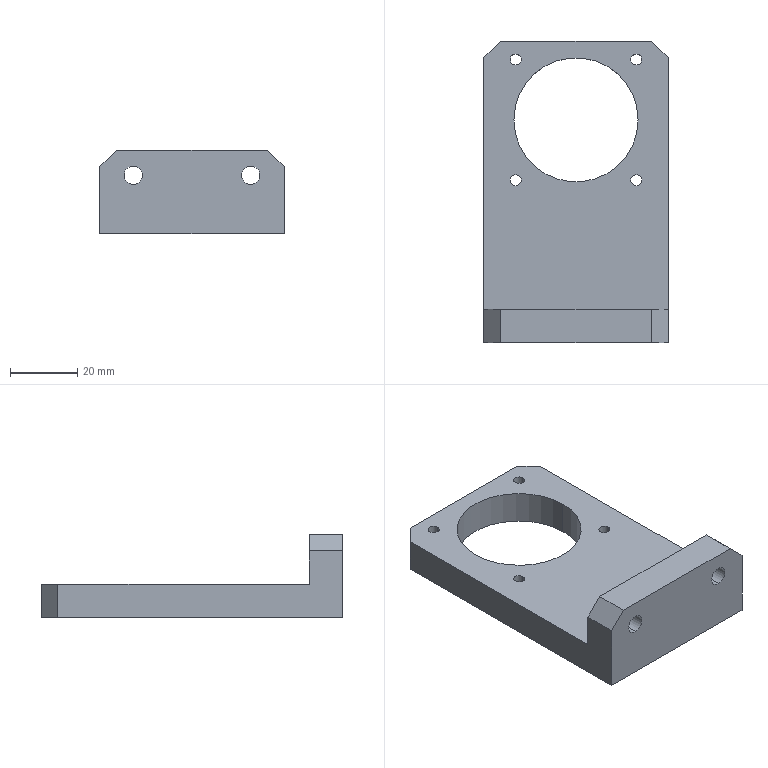Part | NX | features BREP 1 | 1 solid | 26 faces | box 55 x 90 x 25 mm | volume 45681 mm3 | cylinder 14 | plane 12 | commonest cylinder face diameters 3.3 x8 5.5 x4 37 x2
STEP:
#1=CARTESIAN_POINT('',(17.347,3.533,10.));
#2=VERTEX_POINT('',#1);
#3=CARTESIAN_POINT('',(-19.653,3.533,10.));
#4=VERTEX_POINT('',#3);
#5=CARTESIAN_POINT('',(-1.153,3.533,10.));
#6=DIRECTION('',(0.,0.,-1.));
#7=DIRECTION('',(-1.,0.,0.));
#8=AXIS2_PLACEMENT_3D('',#5,#6,#7);
#9=CIRCLE('',#8,18.5);
#10=EDGE_CURVE('',#2,#4,#9,.T.);
#11=ORIENTED_EDGE('',*,*,#10,.F.);
#12=CARTESIAN_POINT('',(17.347,3.533,0.));
#13=VERTEX_POINT('',#12);
#14=CARTESIAN_POINT('',(17.347,3.533,25.));
#15=DIRECTION('',(0.,0.,-1.));
#16=VECTOR('',#15,1000.);
#17=LINE('',#14,#16);
#18=EDGE_CURVE('',#2,#13,#17,.T.);
#19=ORIENTED_EDGE('',*,*,#18,.T.);
#20=CARTESIAN_POINT('',(-19.653,3.533,0.));
#21=VERTEX_POINT('',#20);
#22=CARTESIAN_POINT('',(-1.153,3.533,0.));
#23=DIRECTION('',(0.,0.,-1.));
#24=DIRECTION('',(-1.,0.,0.));
#25=AXIS2_PLACEMENT_3D('',#22,#23,#24);
#26=CIRCLE('',#25,18.5);
#27=EDGE_CURVE('',#13,#21,#26,.T.);
#28=ORIENTED_EDGE('',*,*,#27,.T.);
#29=CARTESIAN_POINT('',(-19.653,3.533,25.));
#30=DIRECTION('',(0.,0.,-1.));
#31=VECTOR('',#30,1000.);
#32=LINE('',#29,#31);
#33=EDGE_CURVE('',#4,#21,#32,.T.);
#34=ORIENTED_EDGE('',*,*,#33,.F.);
#35=EDGE_LOOP('',(#11,#19,#28,#34));
#36=FACE_BOUND('',#35,.T.);
#37=CARTESIAN_POINT('',(-1.153,3.533,25.));
#38=DIRECTION('',(0.,0.,-1.));
#39=DIRECTION('',(-1.,0.,0.));
#40=AXIS2_PLACEMENT_3D('',#37,#38,#39);
#41=CYLINDRICAL_SURFACE('',#40,18.5);
#42=ADVANCED_FACE('',(#36),#41,.F.);
#43=CARTESIAN_POINT('',(18.497,-14.467,0.));
#44=VERTEX_POINT('',#43);
#45=CARTESIAN_POINT('',(15.197,-14.467,0.));
#46=VERTEX_POINT('',#45);
#47=CARTESIAN_POINT('',(16.847,-14.467,0.));
#48=DIRECTION('',(0.,0.,-1.));
#49=DIRECTION('',(1.,0.,0.));
#50=AXIS2_PLACEMENT_3D('',#47,#48,#49);
#51=CIRCLE('',#50,1.65);
#52=EDGE_CURVE('',#44,#46,#51,.T.);
#53=ORIENTED_EDGE('',*,*,#52,.T.);
#54=CARTESIAN_POINT('',(15.197,-14.467,10.));
#55=VERTEX_POINT('',#54);
#56=CARTESIAN_POINT('',(15.197,-14.467,10.));
#57=DIRECTION('',(0.,0.,1.));
#58=VECTOR('',#57,1000.);
#59=LINE('',#56,#58);
#60=EDGE_CURVE('',#55,#46,#59,.F.);
#61=ORIENTED_EDGE('',*,*,#60,.F.);
#62=CARTESIAN_POINT('',(18.497,-14.467,10.));
#63=VERTEX_POINT('',#62);
#64=CARTESIAN_POINT('',(16.847,-14.467,10.));
#65=DIRECTION('',(0.,0.,-1.));
#66=DIRECTION('',(1.,0.,0.));
#67=AXIS2_PLACEMENT_3D('',#64,#65,#66);
#68=CIRCLE('',#67,1.65);
#69=EDGE_CURVE('',#63,#55,#68,.T.);
#70=ORIENTED_EDGE('',*,*,#69,.F.);
#71=CARTESIAN_POINT('',(18.497,-14.467,10.));
#72=DIRECTION('',(0.,0.,1.));
#73=VECTOR('',#72,1000.);
#74=LINE('',#71,#73);
#75=EDGE_CURVE('',#63,#44,#74,.F.);
#76=ORIENTED_EDGE('',*,*,#75,.T.);
#77=EDGE_LOOP('',(#53,#61,#70,#76));
#78=FACE_BOUND('',#77,.T.);
#79=CARTESIAN_POINT('',(16.847,-14.467,10.));
#80=DIRECTION('',(0.,0.,1.));
#81=DIRECTION('',(1.,0.,0.));
#82=AXIS2_PLACEMENT_3D('',#79,#80,#81);
#83=CYLINDRICAL_SURFACE('',#82,1.65);
#84=ADVANCED_FACE('',(#78),#83,.F.);
#85=CARTESIAN_POINT('',(18.497,21.533,0.));
#86=VERTEX_POINT('',#85);
#87=CARTESIAN_POINT('',(15.197,21.533,0.));
#88=VERTEX_POINT('',#87);
#89=CARTESIAN_POINT('',(16.847,21.533,0.));
#90=DIRECTION('',(0.,0.,-1.));
#91=DIRECTION('',(1.,0.,0.));
#92=AXIS2_PLACEMENT_3D('',#89,#90,#91);
#93=CIRCLE('',#92,1.65);
#94=EDGE_CURVE('',#86,#88,#93,.T.);
#95=ORIENTED_EDGE('',*,*,#94,.T.);
#96=CARTESIAN_POINT('',(15.197,21.533,10.));
#97=VERTEX_POINT('',#96);
#98=CARTESIAN_POINT('',(15.197,21.533,10.));
#99=DIRECTION('',(0.,0.,1.));
#100=VECTOR('',#99,1000.);
#101=LINE('',#98,#100);
#102=EDGE_CURVE('',#97,#88,#101,.F.);
#103=ORIENTED_EDGE('',*,*,#102,.F.);
#104=CARTESIAN_POINT('',(18.497,21.533,10.));
#105=VERTEX_POINT('',#104);
#106=CARTESIAN_POINT('',(16.847,21.533,10.));
#107=DIRECTION('',(0.,0.,-1.));
#108=DIRECTION('',(1.,0.,0.));
#109=AXIS2_PLACEMENT_3D('',#106,#107,#108);
#110=CIRCLE('',#109,1.65);
#111=EDGE_CURVE('',#105,#97,#110,.T.);
#112=ORIENTED_EDGE('',*,*,#111,.F.);
#113=CARTESIAN_POINT('',(18.497,21.533,10.));
#114=DIRECTION('',(0.,0.,1.));
#115=VECTOR('',#114,1000.);
#116=LINE('',#113,#115);
#117=EDGE_CURVE('',#105,#86,#116,.F.);
#118=ORIENTED_EDGE('',*,*,#117,.T.);
#119=EDGE_LOOP('',(#95,#103,#112,#118));
#120=FACE_BOUND('',#119,.T.);
#121=CARTESIAN_POINT('',(16.847,21.533,10.));
#122=DIRECTION('',(0.,0.,1.));
#123=DIRECTION('',(1.,0.,0.));
#124=AXIS2_PLACEMENT_3D('',#121,#122,#123);
#125=CYLINDRICAL_SURFACE('',#124,1.65);
#126=ADVANCED_FACE('',(#120),#125,.F.);
#127=CARTESIAN_POINT('',(-17.503,21.533,0.));
#128=VERTEX_POINT('',#127);
#129=CARTESIAN_POINT('',(-20.803,21.533,0.));
#130=VERTEX_POINT('',#129);
#131=CARTESIAN_POINT('',(-19.153,21.533,0.));
#132=DIRECTION('',(0.,0.,-1.));
#133=DIRECTION('',(1.,0.,0.));
#134=AXIS2_PLACEMENT_3D('',#131,#132,#133);
#135=CIRCLE('',#134,1.65);
#136=EDGE_CURVE('',#128,#130,#135,.T.);
#137=ORIENTED_EDGE('',*,*,#136,.T.);
#138=CARTESIAN_POINT('',(-20.803,21.533,10.));
#139=VERTEX_POINT('',#138);
#140=CARTESIAN_POINT('',(-20.803,21.533,10.));
#141=DIRECTION('',(0.,0.,1.));
#142=VECTOR('',#141,1000.);
#143=LINE('',#140,#142);
#144=EDGE_CURVE('',#139,#130,#143,.F.);
#145=ORIENTED_EDGE('',*,*,#144,.F.);
#146=CARTESIAN_POINT('',(-17.503,21.533,10.));
#147=VERTEX_POINT('',#146);
#148=CARTESIAN_POINT('',(-19.153,21.533,10.));
#149=DIRECTION('',(0.,0.,-1.));
#150=DIRECTION('',(1.,0.,0.));
#151=AXIS2_PLACEMENT_3D('',#148,#149,#150);
#152=CIRCLE('',#151,1.65);
#153=EDGE_CURVE('',#147,#139,#152,.T.);
#154=ORIENTED_EDGE('',*,*,#153,.F.);
#155=CARTESIAN_POINT('',(-17.503,21.533,10.));
#156=DIRECTION('',(0.,0.,1.));
#157=VECTOR('',#156,1000.);
#158=LINE('',#155,#157);
#159=EDGE_CURVE('',#147,#128,#158,.F.);
#160=ORIENTED_EDGE('',*,*,#159,.T.);
#161=EDGE_LOOP('',(#137,#145,#154,#160));
#162=FACE_BOUND('',#161,.T.);
#163=CARTESIAN_POINT('',(-19.153,21.533,10.));
#164=DIRECTION('',(0.,0.,1.));
#165=DIRECTION('',(1.,0.,0.));
#166=AXIS2_PLACEMENT_3D('',#163,#164,#165);
#167=CYLINDRICAL_SURFACE('',#166,1.65);
#168=ADVANCED_FACE('',(#162),#167,.F.);
#169=CARTESIAN_POINT('',(-17.503,-14.467,0.));
#170=VERTEX_POINT('',#169);
#171=CARTESIAN_POINT('',(-20.803,-14.467,0.));
#172=VERTEX_POINT('',#171);
#173=CARTESIAN_POINT('',(-19.153,-14.467,0.));
#174=DIRECTION('',(0.,0.,-1.));
#175=DIRECTION('',(1.,0.,0.));
#176=AXIS2_PLACEMENT_3D('',#173,#174,#175);
#177=CIRCLE('',#176,1.65);
#178=EDGE_CURVE('',#170,#172,#177,.T.);
#179=ORIENTED_EDGE('',*,*,#178,.T.);
#180=CARTESIAN_POINT('',(-20.803,-14.467,10.));
#181=VERTEX_POINT('',#180);
#182=CARTESIAN_POINT('',(-20.803,-14.467,10.));
#183=DIRECTION('',(0.,0.,1.));
#184=VECTOR('',#183,1000.);
#185=LINE('',#182,#184);
#186=EDGE_CURVE('',#181,#172,#185,.F.);
#187=ORIENTED_EDGE('',*,*,#186,.F.);
#188=CARTESIAN_POINT('',(-17.503,-14.467,10.));
#189=VERTEX_POINT('',#188);
#190=CARTESIAN_POINT('',(-19.153,-14.467,10.));
#191=DIRECTION('',(0.,0.,-1.));
#192=DIRECTION('',(1.,0.,0.));
#193=AXIS2_PLACEMENT_3D('',#190,#191,#192);
#194=CIRCLE('',#193,1.65);
#195=EDGE_CURVE('',#189,#181,#194,.T.);
#196=ORIENTED_EDGE('',*,*,#195,.F.);
#197=CARTESIAN_POINT('',(-17.503,-14.467,10.));
#198=DIRECTION('',(0.,0.,1.));
#199=VECTOR('',#198,1000.);
#200=LINE('',#197,#199);
#201=EDGE_CURVE('',#189,#170,#200,.F.);
#202=ORIENTED_EDGE('',*,*,#201,.T.);
#203=EDGE_LOOP('',(#179,#187,#196,#202));
#204=FACE_BOUND('',#203,.T.);
#205=CARTESIAN_POINT('',(-19.153,-14.467,10.));
#206=DIRECTION('',(0.,0.,1.));
#207=DIRECTION('',(1.,0.,0.));
#208=AXIS2_PLACEMENT_3D('',#205,#206,#207);
#209=CYLINDRICAL_SURFACE('',#208,1.65);
#210=ADVANCED_FACE('',(#204),#209,.F.);
#211=CARTESIAN_POINT('',(-18.653,-62.967,20.25));
#212=VERTEX_POINT('',#211);
#213=CARTESIAN_POINT('',(-18.653,-62.967,14.75));
#214=VERTEX_POINT('',#213);
#215=CARTESIAN_POINT('',(-18.653,-62.967,17.5));
#216=DIRECTION('',(0.,-1.,0.));
#217=DIRECTION('',(0.,0.,1.));
#218=AXIS2_PLACEMENT_3D('',#215,#216,#217);
#219=CIRCLE('',#218,2.75);
#220=EDGE_CURVE('',#212,#214,#219,.T.);
#221=ORIENTED_EDGE('',*,*,#220,.T.);
#222=CARTESIAN_POINT('',(-18.653,-52.967,14.75));
#223=VERTEX_POINT('',#222);
#224=CARTESIAN_POINT('',(-18.653,-62.967,14.75));
#225=DIRECTION('',(0.,1.,0.));
#226=VECTOR('',#225,1000.);
#227=LINE('',#224,#226);
#228=EDGE_CURVE('',#223,#214,#227,.F.);
#229=ORIENTED_EDGE('',*,*,#228,.F.);
#230=CARTESIAN_POINT('',(-18.653,-52.967,20.25));
#231=VERTEX_POINT('',#230);
#232=CARTESIAN_POINT('',(-18.653,-52.967,17.5));
#233=DIRECTION('',(0.,-1.,0.));
#234=DIRECTION('',(0.,0.,1.));
#235=AXIS2_PLACEMENT_3D('',#232,#233,#234);
#236=CIRCLE('',#235,2.75);
#237=EDGE_CURVE('',#231,#223,#236,.T.);
#238=ORIENTED_EDGE('',*,*,#237,.F.);
#239=CARTESIAN_POINT('',(-18.653,-62.967,20.25));
#240=DIRECTION('',(0.,1.,0.));
#241=VECTOR('',#240,1000.);
#242=LINE('',#239,#241);
#243=EDGE_CURVE('',#231,#212,#242,.F.);
#244=ORIENTED_EDGE('',*,*,#243,.T.);
#245=EDGE_LOOP('',(#221,#229,#238,#244));
#246=FACE_BOUND('',#245,.T.);
#247=CARTESIAN_POINT('',(-18.653,-62.967,17.5));
#248=DIRECTION('',(0.,1.,0.));
#249=DIRECTION('',(0.,0.,1.));
#250=AXIS2_PLACEMENT_3D('',#247,#248,#249);
#251=CYLINDRICAL_SURFACE('',#250,2.75);
#252=ADVANCED_FACE('',(#246),#251,.F.);
#253=CARTESIAN_POINT('',(16.347,-62.967,20.25));
#254=VERTEX_POINT('',#253);
#255=CARTESIAN_POINT('',(16.347,-62.967,14.75));
#256=VERTEX_POINT('',#255);
#257=CARTESIAN_POINT('',(16.347,-62.967,17.5));
#258=DIRECTION('',(0.,-1.,0.));
#259=DIRECTION('',(0.,0.,1.));
#260=AXIS2_PLACEMENT_3D('',#257,#258,#259);
#261=CIRCLE('',#260,2.75);
#262=EDGE_CURVE('',#254,#256,#261,.T.);
#263=ORIENTED_EDGE('',*,*,#262,.T.);
#264=CARTESIAN_POINT('',(16.347,-52.967,14.75));
#265=VERTEX_POINT('',#264);
#266=CARTESIAN_POINT('',(16.347,-62.967,14.75));
#267=DIRECTION('',(0.,1.,0.));
#268=VECTOR('',#267,1000.);
#269=LINE('',#266,#268);
#270=EDGE_CURVE('',#265,#256,#269,.F.);
#271=ORIENTED_EDGE('',*,*,#270,.F.);
#272=CARTESIAN_POINT('',(16.347,-52.967,20.25));
#273=VERTEX_POINT('',#272);
#274=CARTESIAN_POINT('',(16.347,-52.967,17.5));
#275=DIRECTION('',(0.,-1.,0.));
#276=DIRECTION('',(0.,0.,1.));
#277=AXIS2_PLACEMENT_3D('',#274,#275,#276);
#278=CIRCLE('',#277,2.75);
#279=EDGE_CURVE('',#273,#265,#278,.T.);
#280=ORIENTED_EDGE('',*,*,#279,.F.);
#281=CARTESIAN_POINT('',(16.347,-62.967,20.25));
#282=DIRECTION('',(0.,1.,0.));
#283=VECTOR('',#282,1000.);
#284=LINE('',#281,#283);
#285=EDGE_CURVE('',#273,#254,#284,.F.);
#286=ORIENTED_EDGE('',*,*,#285,.T.);
#287=EDGE_LOOP('',(#263,#271,#280,#286));
#288=FACE_BOUND('',#287,.T.);
#289=CARTESIAN_POINT('',(16.347,-62.967,17.5));
#290=DIRECTION('',(0.,1.,0.));
#291=DIRECTION('',(0.,0.,1.));
#292=AXIS2_PLACEMENT_3D('',#289,#290,#291);
#293=CYLINDRICAL_SURFACE('',#292,2.75);
#294=ADVANCED_FACE('',(#288),#293,.F.);
#295=CARTESIAN_POINT('',(26.347,22.033,0.));
#296=VERTEX_POINT('',#295);
#297=CARTESIAN_POINT('',(21.347,27.033,0.));
#298=VERTEX_POINT('',#297);
#299=CARTESIAN_POINT('',(26.347,22.033,0.));
#300=DIRECTION('',(-0.7071,0.7071,0.));
#301=VECTOR('',#300,1000.);
#302=LINE('',#299,#301);
#303=EDGE_CURVE('',#296,#298,#302,.T.);
#304=ORIENTED_EDGE('',*,*,#303,.F.);
#305=CARTESIAN_POINT('',(26.347,-62.967,0.));
#306=VERTEX_POINT('',#305);
#307=CARTESIAN_POINT('',(26.347,-62.967,0.));
#308=DIRECTION('',(0.,1.,0.));
#309=VECTOR('',#308,1000.);
#310=LINE('',#307,#309);
#311=EDGE_CURVE('',#306,#296,#310,.T.);
#312=ORIENTED_EDGE('',*,*,#311,.F.);
#313=CARTESIAN_POINT('',(-28.653,-62.967,0.));
#314=VERTEX_POINT('',#313);
#315=CARTESIAN_POINT('',(-28.653,-62.967,0.));
#316=DIRECTION('',(1.,0.,0.));
#317=VECTOR('',#316,1000.);
#318=LINE('',#315,#317);
#319=EDGE_CURVE('',#314,#306,#318,.T.);
#320=ORIENTED_EDGE('',*,*,#319,.F.);
#321=CARTESIAN_POINT('',(-28.653,22.033,0.));
#322=VERTEX_POINT('',#321);
#323=CARTESIAN_POINT('',(-28.653,-62.967,0.));
#324=DIRECTION('',(0.,-1.,0.));
#325=VECTOR('',#324,1000.);
#326=LINE('',#323,#325);
#327=EDGE_CURVE('',#322,#314,#326,.T.);
#328=ORIENTED_EDGE('',*,*,#327,.F.);
#329=CARTESIAN_POINT('',(-23.653,27.033,0.));
#330=VERTEX_POINT('',#329);
#331=CARTESIAN_POINT('',(-23.653,27.033,0.));
#332=DIRECTION('',(-0.7071,-0.7071,0.));
#333=VECTOR('',#332,1000.);
#334=LINE('',#331,#333);
#335=EDGE_CURVE('',#330,#322,#334,.T.);
#336=ORIENTED_EDGE('',*,*,#335,.F.);
#337=CARTESIAN_POINT('',(-28.653,27.033,0.));
#338=DIRECTION('',(-1.,0.,0.));
#339=VECTOR('',#338,1000.);
#340=LINE('',#337,#339);
#341=EDGE_CURVE('',#298,#330,#340,.T.);
#342=ORIENTED_EDGE('',*,*,#341,.F.);
#343=EDGE_LOOP('',(#304,#312,#320,#328,#336,#342));
#344=FACE_BOUND('',#343,.T.);
#345=CARTESIAN_POINT('',(-1.153,3.533,0.));
#346=DIRECTION('',(0.,0.,-1.));
#347=DIRECTION('',(-1.,0.,0.));
#348=AXIS2_PLACEMENT_3D('',#345,#346,#347);
#349=CIRCLE('',#348,18.5);
#350=EDGE_CURVE('',#21,#13,#349,.T.);
#351=ORIENTED_EDGE('',*,*,#350,.F.);
#352=ORIENTED_EDGE('',*,*,#27,.F.);
#353=EDGE_LOOP('',(#351,#352));
#354=FACE_BOUND('',#353,.T.);
#355=ORIENTED_EDGE('',*,*,#52,.F.);
#356=CARTESIAN_POINT('',(16.847,-14.467,0.));
#357=DIRECTION('',(0.,0.,-1.));
#358=DIRECTION('',(1.,0.,0.));
#359=AXIS2_PLACEMENT_3D('',#356,#357,#358);
#360=CIRCLE('',#359,1.65);
#361=EDGE_CURVE('',#46,#44,#360,.T.);
#362=ORIENTED_EDGE('',*,*,#361,.F.);
#363=EDGE_LOOP('',(#355,#362));
#364=FACE_BOUND('',#363,.T.);
#365=ORIENTED_EDGE('',*,*,#94,.F.);
#366=CARTESIAN_POINT('',(16.847,21.533,0.));
#367=DIRECTION('',(0.,0.,-1.));
#368=DIRECTION('',(1.,0.,0.));
#369=AXIS2_PLACEMENT_3D('',#366,#367,#368);
#370=CIRCLE('',#369,1.65);
#371=EDGE_CURVE('',#88,#86,#370,.T.);
#372=ORIENTED_EDGE('',*,*,#371,.F.);
#373=EDGE_LOOP('',(#365,#372));
#374=FACE_BOUND('',#373,.T.);
#375=ORIENTED_EDGE('',*,*,#136,.F.);
#376=CARTESIAN_POINT('',(-19.153,21.533,0.));
#377=DIRECTION('',(0.,0.,-1.));
#378=DIRECTION('',(1.,0.,0.));
#379=AXIS2_PLACEMENT_3D('',#376,#377,#378);
#380=CIRCLE('',#379,1.65);
#381=EDGE_CURVE('',#130,#128,#380,.T.);
#382=ORIENTED_EDGE('',*,*,#381,.F.);
#383=EDGE_LOOP('',(#375,#382));
#384=FACE_BOUND('',#383,.T.);
#385=ORIENTED_EDGE('',*,*,#178,.F.);
#386=CARTESIAN_POINT('',(-19.153,-14.467,0.));
#387=DIRECTION('',(0.,0.,-1.));
#388=DIRECTION('',(1.,0.,0.));
#389=AXIS2_PLACEMENT_3D('',#386,#387,#388);
#390=CIRCLE('',#389,1.65);
#391=EDGE_CURVE('',#172,#170,#390,.T.);
#392=ORIENTED_EDGE('',*,*,#391,.F.);
#393=EDGE_LOOP('',(#385,#392));
#394=FACE_BOUND('',#393,.T.);
#395=CARTESIAN_POINT('',(-28.653,-62.967,0.));
#396=DIRECTION('',(0.,0.,1.));
#397=DIRECTION('',(1.,0.,0.));
#398=AXIS2_PLACEMENT_3D('',#395,#396,#397);
#399=PLANE('',#398);
#400=ADVANCED_FACE('',(#344,#354,#364,#374,#384,#394),#399,.F.);
#401=CARTESIAN_POINT('',(21.347,27.033,10.));
#402=VERTEX_POINT('',#401);
#403=CARTESIAN_POINT('',(21.347,27.033,10.));
#404=DIRECTION('',(0.,0.,1.));
#405=VECTOR('',#404,1000.);
#406=LINE('',#403,#405);
#407=EDGE_CURVE('',#298,#402,#406,.T.);
#408=ORIENTED_EDGE('',*,*,#407,.F.);
#409=ORIENTED_EDGE('',*,*,#341,.T.);
#410=CARTESIAN_POINT('',(-23.653,27.033,10.));
#411=VERTEX_POINT('',#410);
#412=CARTESIAN_POINT('',(-23.653,27.033,10.));
#413=DIRECTION('',(0.,0.,-1.));
#414=VECTOR('',#413,1000.);
#415=LINE('',#412,#414);
#416=EDGE_CURVE('',#411,#330,#415,.T.);
#417=ORIENTED_EDGE('',*,*,#416,.F.);
#418=CARTESIAN_POINT('',(-28.653,27.033,10.));
#419=DIRECTION('',(-1.,0.,0.));
#420=VECTOR('',#419,1000.);
#421=LINE('',#418,#420);
#422=EDGE_CURVE('',#402,#411,#421,.T.);
#423=ORIENTED_EDGE('',*,*,#422,.F.);
#424=EDGE_LOOP('',(#408,#409,#417,#423));
#425=FACE_BOUND('',#424,.T.);
#426=CARTESIAN_POINT('',(-28.653,27.033,10.));
#427=DIRECTION('',(0.,-1.,0.));
#428=DIRECTION('',(0.,0.,-1.));
#429=AXIS2_PLACEMENT_3D('',#426,#427,#428);
#430=PLANE('',#429);
#431=ADVANCED_FACE('',(#425),#430,.F.);
#432=CARTESIAN_POINT('',(26.347,22.033,10.));
#433=VERTEX_POINT('',#432);
#434=CARTESIAN_POINT('',(26.347,22.033,10.));
#435=DIRECTION('',(0.,0.,1.));
#436=VECTOR('',#435,1000.);
#437=LINE('',#434,#436);
#438=EDGE_CURVE('',#296,#433,#437,.T.);
#439=ORIENTED_EDGE('',*,*,#438,.F.);
#440=ORIENTED_EDGE('',*,*,#303,.T.);
#441=ORIENTED_EDGE('',*,*,#407,.T.);
#442=CARTESIAN_POINT('',(21.347,27.033,10.));
#443=DIRECTION('',(-0.7071,0.7071,0.));
#444=VECTOR('',#443,1000.);
#445=LINE('',#442,#444);
#446=EDGE_CURVE('',#433,#402,#445,.T.);
#447=ORIENTED_EDGE('',*,*,#446,.F.);
#448=EDGE_LOOP('',(#439,#440,#441,#447));
#449=FACE_BOUND('',#448,.T.);
#450=CARTESIAN_POINT('',(21.347,27.033,10.));
#451=DIRECTION('',(-0.7071,-0.7071,0.));
#452=DIRECTION('',(-0.7071,0.7071,0.));
#453=AXIS2_PLACEMENT_3D('',#450,#451,#452);
#454=PLANE('',#453);
#455=ADVANCED_FACE('',(#449),#454,.F.);
#456=CARTESIAN_POINT('',(26.347,-62.967,20.));
#457=VERTEX_POINT('',#456);
#458=CARTESIAN_POINT('',(26.347,-52.967,20.));
#459=VERTEX_POINT('',#458);
#460=CARTESIAN_POINT('',(26.347,27.033,20.));
#461=DIRECTION('',(0.,1.,0.));
#462=VECTOR('',#461,1000.);
#463=LINE('',#460,#462);
#464=EDGE_CURVE('',#457,#459,#463,.T.);
#465=ORIENTED_EDGE('',*,*,#464,.F.);
#466=CARTESIAN_POINT('',(26.347,-62.967,10.));
#467=DIRECTION('',(0.,0.,1.));
#468=VECTOR('',#467,1000.);
#469=LINE('',#466,#468);
#470=EDGE_CURVE('',#306,#457,#469,.T.);
#471=ORIENTED_EDGE('',*,*,#470,.F.);
#472=ORIENTED_EDGE('',*,*,#311,.T.);
#473=ORIENTED_EDGE('',*,*,#438,.T.);
#474=CARTESIAN_POINT('',(26.347,-52.967,10.));
#475=VERTEX_POINT('',#474);
#476=CARTESIAN_POINT('',(26.347,27.033,10.));
#477=DIRECTION('',(0.,1.,0.));
#478=VECTOR('',#477,1000.);
#479=LINE('',#476,#478);
#480=EDGE_CURVE('',#475,#433,#479,.T.);
#481=ORIENTED_EDGE('',*,*,#480,.F.);
#482=CARTESIAN_POINT('',(26.347,-52.967,10.));
#483=DIRECTION('',(0.,0.,-1.));
#484=VECTOR('',#483,1000.);
#485=LINE('',#482,#484);
#486=EDGE_CURVE('',#459,#475,#485,.T.);
#487=ORIENTED_EDGE('',*,*,#486,.F.);
#488=EDGE_LOOP('',(#465,#471,#472,#473,#481,#487));
#489=FACE_BOUND('',#488,.T.);
#490=CARTESIAN_POINT('',(26.347,27.033,10.));
#491=DIRECTION('',(-1.,0.,0.));
#492=DIRECTION('',(0.,1.,0.));
#493=AXIS2_PLACEMENT_3D('',#490,#491,#492);
#494=PLANE('',#493);
#495=ADVANCED_FACE('',(#489),#494,.F.);
#496=CARTESIAN_POINT('',(-28.653,-62.967,20.));
#497=VERTEX_POINT('',#496);
#498=CARTESIAN_POINT('',(-23.653,-62.967,25.));
#499=VERTEX_POINT('',#498);
#500=CARTESIAN_POINT('',(-28.653,-62.967,20.));
#501=DIRECTION('',(0.7071,0.,0.7071));
#502=VECTOR('',#501,1000.);
#503=LINE('',#500,#502);
#504=EDGE_CURVE('',#497,#499,#503,.T.);
#505=ORIENTED_EDGE('',*,*,#504,.F.);
#506=CARTESIAN_POINT('',(-28.653,-62.967,10.));
#507=DIRECTION('',(0.,0.,1.));
#508=VECTOR('',#507,1000.);
#509=LINE('',#506,#508);
#510=EDGE_CURVE('',#314,#497,#509,.T.);
#511=ORIENTED_EDGE('',*,*,#510,.F.);
#512=ORIENTED_EDGE('',*,*,#319,.T.);
#513=ORIENTED_EDGE('',*,*,#470,.T.);
#514=CARTESIAN_POINT('',(21.347,-62.967,25.));
#515=VERTEX_POINT('',#514);
#516=CARTESIAN_POINT('',(21.347,-62.967,25.));
#517=DIRECTION('',(0.7071,0.,-0.7071));
#518=VECTOR('',#517,1000.);
#519=LINE('',#516,#518);
#520=EDGE_CURVE('',#515,#457,#519,.T.);
#521=ORIENTED_EDGE('',*,*,#520,.F.);
#522=CARTESIAN_POINT('',(-28.653,-62.967,25.));
#523=DIRECTION('',(1.,0.,0.));
#524=VECTOR('',#523,1000.);
#525=LINE('',#522,#524);
#526=EDGE_CURVE('',#499,#515,#525,.T.);
#527=ORIENTED_EDGE('',*,*,#526,.F.);
#528=EDGE_LOOP('',(#505,#511,#512,#513,#521,#527));
#529=FACE_BOUND('',#528,.T.);
#530=ORIENTED_EDGE('',*,*,#220,.F.);
#531=CARTESIAN_POINT('',(-18.653,-62.967,17.5));
#532=DIRECTION('',(0.,-1.,0.));
#533=DIRECTION('',(0.,0.,1.));
#534=AXIS2_PLACEMENT_3D('',#531,#532,#533);
#535=CIRCLE('',#534,2.75);
#536=EDGE_CURVE('',#214,#212,#535,.T.);
#537=ORIENTED_EDGE('',*,*,#536,.F.);
#538=EDGE_LOOP('',(#530,#537));
#539=FACE_BOUND('',#538,.T.);
#540=ORIENTED_EDGE('',*,*,#262,.F.);
#541=CARTESIAN_POINT('',(16.347,-62.967,17.5));
#542=DIRECTION('',(0.,-1.,0.));
#543=DIRECTION('',(0.,0.,1.));
#544=AXIS2_PLACEMENT_3D('',#541,#542,#543);
#545=CIRCLE('',#544,2.75);
#546=EDGE_CURVE('',#256,#254,#545,.T.);
#547=ORIENTED_EDGE('',*,*,#546,.F.);
#548=EDGE_LOOP('',(#540,#547));
#549=FACE_BOUND('',#548,.T.);
#550=CARTESIAN_POINT('',(-28.653,-62.967,10.));
#551=DIRECTION('',(0.,1.,0.));
#552=DIRECTION('',(1.,0.,0.));
#553=AXIS2_PLACEMENT_3D('',#550,#551,#552);
#554=PLANE('',#553);
#555=ADVANCED_FACE('',(#529,#539,#549),#554,.F.);
#556=CARTESIAN_POINT('',(-28.653,-52.967,20.));
#557=VERTEX_POINT('',#556);
#558=CARTESIAN_POINT('',(-28.653,27.033,20.));
#559=DIRECTION('',(0.,-1.,0.));
#560=VECTOR('',#559,1000.);
#561=LINE('',#558,#560);
#562=EDGE_CURVE('',#557,#497,#561,.T.);
#563=ORIENTED_EDGE('',*,*,#562,.F.);
#564=CARTESIAN_POINT('',(-28.653,-52.967,10.));
#565=VERTEX_POINT('',#564);
#566=CARTESIAN_POINT('',(-28.653,-52.967,10.));
#567=DIRECTION('',(0.,0.,1.));
#568=VECTOR('',#567,1000.);
#569=LINE('',#566,#568);
#570=EDGE_CURVE('',#565,#557,#569,.T.);
#571=ORIENTED_EDGE('',*,*,#570,.F.);
#572=CARTESIAN_POINT('',(-28.653,22.033,10.));
#573=VERTEX_POINT('',#572);
#574=CARTESIAN_POINT('',(-28.653,27.033,10.));
#575=DIRECTION('',(0.,-1.,0.));
#576=VECTOR('',#575,1000.);
#577=LINE('',#574,#576);
#578=EDGE_CURVE('',#573,#565,#577,.T.);
#579=ORIENTED_EDGE('',*,*,#578,.F.);
#580=CARTESIAN_POINT('',(-28.653,22.033,10.));
#581=DIRECTION('',(0.,0.,1.));
#582=VECTOR('',#581,1000.);
#583=LINE('',#580,#582);
#584=EDGE_CURVE('',#322,#573,#583,.T.);
#585=ORIENTED_EDGE('',*,*,#584,.F.);
#586=ORIENTED_EDGE('',*,*,#327,.T.);
#587=ORIENTED_EDGE('',*,*,#510,.T.);
#588=EDGE_LOOP('',(#563,#571,#579,#585,#586,#587));
#589=FACE_BOUND('',#588,.T.);
#590=CARTESIAN_POINT('',(-28.653,27.033,10.));
#591=DIRECTION('',(1.,0.,0.));
#592=DIRECTION('',(0.,1.,0.));
#593=AXIS2_PLACEMENT_3D('',#590,#591,#592);
#594=PLANE('',#593);
#595=ADVANCED_FACE('',(#589),#594,.F.);
#596=ORIENTED_EDGE('',*,*,#416,.T.);
#597=ORIENTED_EDGE('',*,*,#335,.T.);
#598=ORIENTED_EDGE('',*,*,#584,.T.);
#599=CARTESIAN_POINT('',(-28.653,22.033,10.));
#600=DIRECTION('',(-0.7071,-0.7071,0.));
#601=VECTOR('',#600,1000.);
#602=LINE('',#599,#601);
#603=EDGE_CURVE('',#411,#573,#602,.T.);
#604=ORIENTED_EDGE('',*,*,#603,.F.);
#605=EDGE_LOOP('',(#596,#597,#598,#604));
#606=FACE_BOUND('',#605,.T.);
#607=CARTESIAN_POINT('',(-28.653,22.033,10.));
#608=DIRECTION('',(0.7071,-0.7071,0.));
#609=DIRECTION('',(0.,0.,-1.));
#610=AXIS2_PLACEMENT_3D('',#607,#608,#609);
#611=PLANE('',#610);
#612=ADVANCED_FACE('',(#606),#611,.F.);
#613=ORIENTED_EDGE('',*,*,#18,.F.);
#614=CARTESIAN_POINT('',(-1.153,3.533,10.));
#615=DIRECTION('',(0.,0.,-1.));
#616=DIRECTION('',(-1.,0.,0.));
#617=AXIS2_PLACEMENT_3D('',#614,#615,#616);
#618=CIRCLE('',#617,18.5);
#619=EDGE_CURVE('',#4,#2,#618,.T.);
#620=ORIENTED_EDGE('',*,*,#619,.F.);
#621=ORIENTED_EDGE('',*,*,#33,.T.);
#622=ORIENTED_EDGE('',*,*,#350,.T.);
#623=EDGE_LOOP('',(#613,#620,#621,#622));
#624=FACE_BOUND('',#623,.T.);
#625=CARTESIAN_POINT('',(-1.153,3.533,25.));
#626=DIRECTION('',(0.,0.,-1.));
#627=DIRECTION('',(-1.,0.,0.));
#628=AXIS2_PLACEMENT_3D('',#625,#626,#627);
#629=CYLINDRICAL_SURFACE('',#628,18.5);
#630=ADVANCED_FACE('',(#624),#629,.F.);
#631=ORIENTED_EDGE('',*,*,#60,.T.);
#632=ORIENTED_EDGE('',*,*,#361,.T.);
#633=ORIENTED_EDGE('',*,*,#75,.F.);
#634=CARTESIAN_POINT('',(16.847,-14.467,10.));
#635=DIRECTION('',(0.,0.,-1.));
#636=DIRECTION('',(1.,0.,0.));
#637=AXIS2_PLACEMENT_3D('',#634,#635,#636);
#638=CIRCLE('',#637,1.65);
#639=EDGE_CURVE('',#55,#63,#638,.T.);
#640=ORIENTED_EDGE('',*,*,#639,.F.);
#641=EDGE_LOOP('',(#631,#632,#633,#640));
#642=FACE_BOUND('',#641,.T.);
#643=CARTESIAN_POINT('',(16.847,-14.467,10.));
#644=DIRECTION('',(0.,0.,1.));
#645=DIRECTION('',(1.,0.,0.));
#646=AXIS2_PLACEMENT_3D('',#643,#644,#645);
#647=CYLINDRICAL_SURFACE('',#646,1.65);
#648=ADVANCED_FACE('',(#642),#647,.F.);
#649=ORIENTED_EDGE('',*,*,#102,.T.);
#650=ORIENTED_EDGE('',*,*,#371,.T.);
#651=ORIENTED_EDGE('',*,*,#117,.F.);
#652=CARTESIAN_POINT('',(16.847,21.533,10.));
#653=DIRECTION('',(0.,0.,-1.));
#654=DIRECTION('',(1.,0.,0.));
#655=AXIS2_PLACEMENT_3D('',#652,#653,#654);
#656=CIRCLE('',#655,1.65);
#657=EDGE_CURVE('',#97,#105,#656,.T.);
#658=ORIENTED_EDGE('',*,*,#657,.F.);
#659=EDGE_LOOP('',(#649,#650,#651,#658));
#660=FACE_BOUND('',#659,.T.);
#661=CARTESIAN_POINT('',(16.847,21.533,10.));
#662=DIRECTION('',(0.,0.,1.));
#663=DIRECTION('',(1.,0.,0.));
#664=AXIS2_PLACEMENT_3D('',#661,#662,#663);
#665=CYLINDRICAL_SURFACE('',#664,1.65);
#666=ADVANCED_FACE('',(#660),#665,.F.);
#667=ORIENTED_EDGE('',*,*,#144,.T.);
#668=ORIENTED_EDGE('',*,*,#381,.T.);
#669=ORIENTED_EDGE('',*,*,#159,.F.);
#670=CARTESIAN_POINT('',(-19.153,21.533,10.));
#671=DIRECTION('',(0.,0.,-1.));
#672=DIRECTION('',(1.,0.,0.));
#673=AXIS2_PLACEMENT_3D('',#670,#671,#672);
#674=CIRCLE('',#673,1.65);
#675=EDGE_CURVE('',#139,#147,#674,.T.);
#676=ORIENTED_EDGE('',*,*,#675,.F.);
#677=EDGE_LOOP('',(#667,#668,#669,#676));
#678=FACE_BOUND('',#677,.T.);
#679=CARTESIAN_POINT('',(-19.153,21.533,10.));
#680=DIRECTION('',(0.,0.,1.));
#681=DIRECTION('',(1.,0.,0.));
#682=AXIS2_PLACEMENT_3D('',#679,#680,#681);
#683=CYLINDRICAL_SURFACE('',#682,1.65);
#684=ADVANCED_FACE('',(#678),#683,.F.);
#685=ORIENTED_EDGE('',*,*,#186,.T.);
#686=ORIENTED_EDGE('',*,*,#391,.T.);
#687=ORIENTED_EDGE('',*,*,#201,.F.);
#688=CARTESIAN_POINT('',(-19.153,-14.467,10.));
#689=DIRECTION('',(0.,0.,-1.));
#690=DIRECTION('',(1.,0.,0.));
#691=AXIS2_PLACEMENT_3D('',#688,#689,#690);
#692=CIRCLE('',#691,1.65);
#693=EDGE_CURVE('',#181,#189,#692,.T.);
#694=ORIENTED_EDGE('',*,*,#693,.F.);
#695=EDGE_LOOP('',(#685,#686,#687,#694));
#696=FACE_BOUND('',#695,.T.);
#697=CARTESIAN_POINT('',(-19.153,-14.467,10.));
#698=DIRECTION('',(0.,0.,1.));
#699=DIRECTION('',(1.,0.,0.));
#700=AXIS2_PLACEMENT_3D('',#697,#698,#699);
#701=CYLINDRICAL_SURFACE('',#700,1.65);
#702=ADVANCED_FACE('',(#696),#701,.F.);
#703=ORIENTED_EDGE('',*,*,#578,.T.);
#704=CARTESIAN_POINT('',(-28.653,-52.967,10.));
#705=DIRECTION('',(1.,0.,0.));
#706=VECTOR('',#705,1000.);
#707=LINE('',#704,#706);
#708=EDGE_CURVE('',#565,#475,#707,.T.);
#709=ORIENTED_EDGE('',*,*,#708,.T.);
#710=ORIENTED_EDGE('',*,*,#480,.T.);
#711=ORIENTED_EDGE('',*,*,#446,.T.);
#712=ORIENTED_EDGE('',*,*,#422,.T.);
#713=ORIENTED_EDGE('',*,*,#603,.T.);
#714=EDGE_LOOP('',(#703,#709,#710,#711,#712,#713));
#715=FACE_BOUND('',#714,.T.);
#716=ORIENTED_EDGE('',*,*,#619,.T.);
#717=ORIENTED_EDGE('',*,*,#10,.T.);
#718=EDGE_LOOP('',(#716,#717));
#719=FACE_BOUND('',#718,.T.);
#720=ORIENTED_EDGE('',*,*,#69,.T.);
#721=ORIENTED_EDGE('',*,*,#639,.T.);
#722=EDGE_LOOP('',(#720,#721));
#723=FACE_BOUND('',#722,.T.);
#724=ORIENTED_EDGE('',*,*,#111,.T.);
#725=ORIENTED_EDGE('',*,*,#657,.T.);
#726=EDGE_LOOP('',(#724,#725));
#727=FACE_BOUND('',#726,.T.);
#728=ORIENTED_EDGE('',*,*,#153,.T.);
#729=ORIENTED_EDGE('',*,*,#675,.T.);
#730=EDGE_LOOP('',(#728,#729));
#731=FACE_BOUND('',#730,.T.);
#732=ORIENTED_EDGE('',*,*,#195,.T.);
#733=ORIENTED_EDGE('',*,*,#693,.T.);
#734=EDGE_LOOP('',(#732,#733));
#735=FACE_BOUND('',#734,.T.);
#736=CARTESIAN_POINT('',(-28.653,-62.967,10.));
#737=DIRECTION('',(0.,0.,1.));
#738=DIRECTION('',(1.,0.,0.));
#739=AXIS2_PLACEMENT_3D('',#736,#737,#738);
#740=PLANE('',#739);
#741=ADVANCED_FACE('',(#715,#719,#723,#727,#731,#735),#740,.T.);
#742=ORIENTED_EDGE('',*,*,#486,.T.);
#743=ORIENTED_EDGE('',*,*,#708,.F.);
#744=ORIENTED_EDGE('',*,*,#570,.T.);
#745=CARTESIAN_POINT('',(-23.653,-52.967,25.));
#746=VERTEX_POINT('',#745);
#747=CARTESIAN_POINT('',(-28.653,-52.967,20.));
#748=DIRECTION('',(0.7071,0.,0.7071));
#749=VECTOR('',#748,1000.);
#750=LINE('',#747,#749);
#751=EDGE_CURVE('',#557,#746,#750,.T.);
#752=ORIENTED_EDGE('',*,*,#751,.T.);
#753=CARTESIAN_POINT('',(21.347,-52.967,25.));
#754=VERTEX_POINT('',#753);
#755=CARTESIAN_POINT('',(44.375,-52.967,25.));
#756=DIRECTION('',(1.,0.,0.));
#757=VECTOR('',#756,1000.);
#758=LINE('',#755,#757);
#759=EDGE_CURVE('',#746,#754,#758,.T.);
#760=ORIENTED_EDGE('',*,*,#759,.T.);
#761=CARTESIAN_POINT('',(21.347,-52.967,25.));
#762=DIRECTION('',(0.7071,0.,-0.7071));
#763=VECTOR('',#762,1000.);
#764=LINE('',#761,#763);
#765=EDGE_CURVE('',#754,#459,#764,.T.);
#766=ORIENTED_EDGE('',*,*,#765,.T.);
#767=EDGE_LOOP('',(#742,#743,#744,#752,#760,#766));
#768=FACE_BOUND('',#767,.T.);
#769=ORIENTED_EDGE('',*,*,#237,.T.);
#770=CARTESIAN_POINT('',(-18.653,-52.967,17.5));
#771=DIRECTION('',(0.,-1.,0.));
#772=DIRECTION('',(0.,0.,1.));
#773=AXIS2_PLACEMENT_3D('',#770,#771,#772);
#774=CIRCLE('',#773,2.75);
#775=EDGE_CURVE('',#223,#231,#774,.T.);
#776=ORIENTED_EDGE('',*,*,#775,.T.);
#777=EDGE_LOOP('',(#769,#776));
#778=FACE_BOUND('',#777,.T.);
#779=ORIENTED_EDGE('',*,*,#279,.T.);
#780=CARTESIAN_POINT('',(16.347,-52.967,17.5));
#781=DIRECTION('',(0.,-1.,0.));
#782=DIRECTION('',(0.,0.,1.));
#783=AXIS2_PLACEMENT_3D('',#780,#781,#782);
#784=CIRCLE('',#783,2.75);
#785=EDGE_CURVE('',#265,#273,#784,.T.);
#786=ORIENTED_EDGE('',*,*,#785,.T.);
#787=EDGE_LOOP('',(#779,#786));
#788=FACE_BOUND('',#787,.T.);
#789=CARTESIAN_POINT('',(44.375,-52.967,10.));
#790=DIRECTION('',(0.,1.,0.));
#791=DIRECTION('',(1.,0.,0.));
#792=AXIS2_PLACEMENT_3D('',#789,#790,#791);
#793=PLANE('',#792);
#794=ADVANCED_FACE('',(#768,#778,#788),#793,.T.);
#795=ORIENTED_EDGE('',*,*,#520,.T.);
#796=ORIENTED_EDGE('',*,*,#464,.T.);
#797=ORIENTED_EDGE('',*,*,#765,.F.);
#798=CARTESIAN_POINT('',(21.347,27.033,25.));
#799=DIRECTION('',(0.,-1.,0.));
#800=VECTOR('',#799,1000.);
#801=LINE('',#798,#800);
#802=EDGE_CURVE('',#754,#515,#801,.T.);
#803=ORIENTED_EDGE('',*,*,#802,.T.);
#804=EDGE_LOOP('',(#795,#796,#797,#803));
#805=FACE_BOUND('',#804,.T.);
#806=CARTESIAN_POINT('',(26.347,27.033,20.));
#807=DIRECTION('',(0.7071,0.,0.7071));
#808=DIRECTION('',(0.,-1.,0.));
#809=AXIS2_PLACEMENT_3D('',#806,#807,#808);
#810=PLANE('',#809);
#811=ADVANCED_FACE('',(#805),#810,.T.);
#812=ORIENTED_EDGE('',*,*,#526,.T.);
#813=ORIENTED_EDGE('',*,*,#802,.F.);
#814=ORIENTED_EDGE('',*,*,#759,.F.);
#815=CARTESIAN_POINT('',(-23.653,-62.967,25.));
#816=DIRECTION('',(0.,-1.,0.));
#817=VECTOR('',#816,1000.);
#818=LINE('',#815,#817);
#819=EDGE_CURVE('',#746,#499,#818,.T.);
#820=ORIENTED_EDGE('',*,*,#819,.T.);
#821=EDGE_LOOP('',(#812,#813,#814,#820));
#822=FACE_BOUND('',#821,.T.);
#823=CARTESIAN_POINT('',(44.375,-62.967,25.));
#824=DIRECTION('',(0.,0.,1.));
#825=DIRECTION('',(1.,0.,0.));
#826=AXIS2_PLACEMENT_3D('',#823,#824,#825);
#827=PLANE('',#826);
#828=ADVANCED_FACE('',(#822),#827,.T.);
#829=ORIENTED_EDGE('',*,*,#751,.F.);
#830=ORIENTED_EDGE('',*,*,#562,.T.);
#831=ORIENTED_EDGE('',*,*,#504,.T.);
#832=ORIENTED_EDGE('',*,*,#819,.F.);
#833=EDGE_LOOP('',(#829,#830,#831,#832));
#834=FACE_BOUND('',#833,.T.);
#835=CARTESIAN_POINT('',(-28.653,27.033,20.));
#836=DIRECTION('',(-0.7071,0.,0.7071));
#837=DIRECTION('',(0.,1.,0.));
#838=AXIS2_PLACEMENT_3D('',#835,#836,#837);
#839=PLANE('',#838);
#840=ADVANCED_FACE('',(#834),#839,.T.);
#841=ORIENTED_EDGE('',*,*,#228,.T.);
#842=ORIENTED_EDGE('',*,*,#536,.T.);
#843=ORIENTED_EDGE('',*,*,#243,.F.);
#844=ORIENTED_EDGE('',*,*,#775,.F.);
#845=EDGE_LOOP('',(#841,#842,#843,#844));
#846=FACE_BOUND('',#845,.T.);
#847=CARTESIAN_POINT('',(-18.653,-62.967,17.5));
#848=DIRECTION('',(0.,1.,0.));
#849=DIRECTION('',(0.,0.,1.));
#850=AXIS2_PLACEMENT_3D('',#847,#848,#849);
#851=CYLINDRICAL_SURFACE('',#850,2.75);
#852=ADVANCED_FACE('',(#846),#851,.F.);
#853=ORIENTED_EDGE('',*,*,#270,.T.);
#854=ORIENTED_EDGE('',*,*,#546,.T.);
#855=ORIENTED_EDGE('',*,*,#285,.F.);
#856=ORIENTED_EDGE('',*,*,#785,.F.);
#857=EDGE_LOOP('',(#853,#854,#855,#856));
#858=FACE_BOUND('',#857,.T.);
#859=CARTESIAN_POINT('',(16.347,-62.967,17.5));
#860=DIRECTION('',(0.,1.,0.));
#861=DIRECTION('',(0.,0.,1.));
#862=AXIS2_PLACEMENT_3D('',#859,#860,#861);
#863=CYLINDRICAL_SURFACE('',#862,2.75);
#864=ADVANCED_FACE('',(#858),#863,.F.);
#865=CLOSED_SHELL('',(#42,#84,#126,#168,#210,#252,#294,#400,#431,#455,#495,#555,#595,#612,#630,#648,#666,#684,#702,#741,#794,#811,#828,#840,#852,#864));
#866=MANIFOLD_SOLID_BREP('',#865);
#867=(LENGTH_UNIT()NAMED_UNIT(*)SI_UNIT(.MILLI.,.METRE.));
#868=UNCERTAINTY_MEASURE_WITH_UNIT(LENGTH_MEASURE(0.00001),#867,'','');
#869=(NAMED_UNIT(*)PLANE_ANGLE_UNIT()SI_UNIT($,.RADIAN.));
#870=(NAMED_UNIT(*)SI_UNIT($,.STERADIAN.)SOLID_ANGLE_UNIT());
#871=(GEOMETRIC_REPRESENTATION_CONTEXT(3)GLOBAL_UNCERTAINTY_ASSIGNED_CONTEXT((#868))GLOBAL_UNIT_ASSIGNED_CONTEXT((#867,#869,#870))REPRESENTATION_CONTEXT('',''));
#872=ADVANCED_BREP_SHAPE_REPRESENTATION('',(#866),#871);